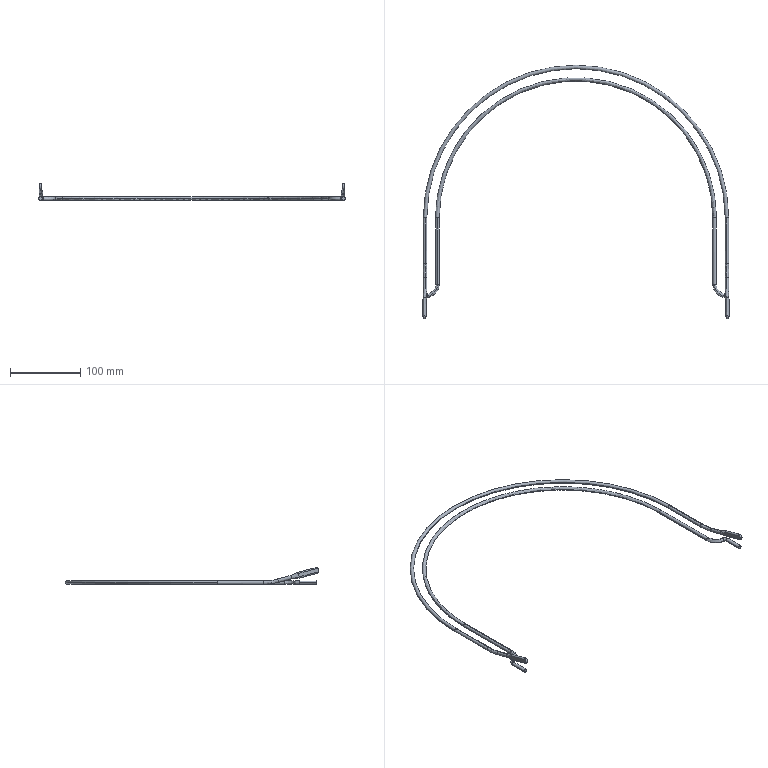Part | SolidWorks | features BaseBody 2 | 2 solids | 67 faces | box 435.2 x 360.06 x 23.767 mm | volume 37382 mm3 | cylinder 33 | spline 18 | plane 14 | torus 2 | commonest cylinder face diameters 5 x24 3.4 x6 8.5 x3